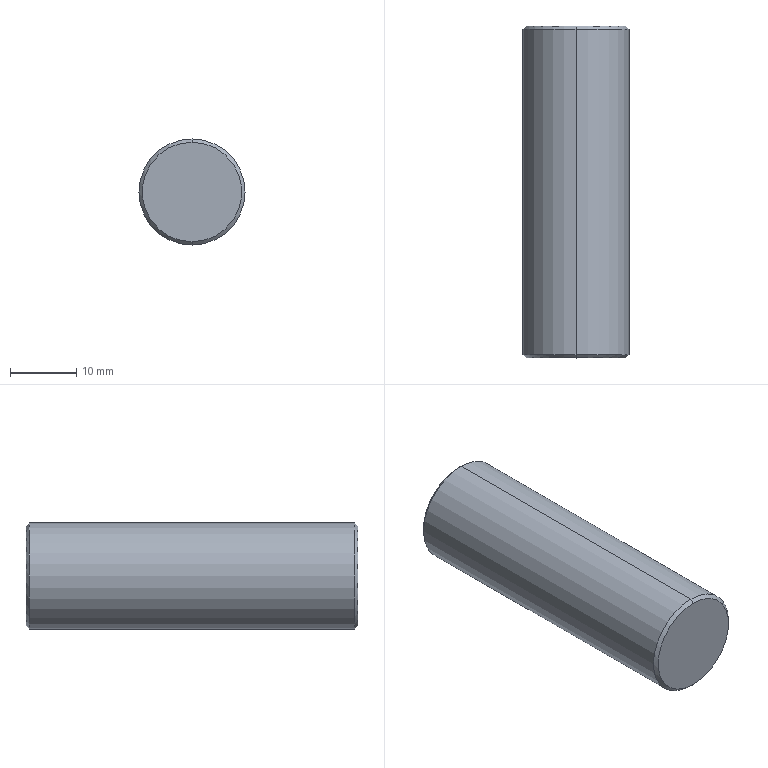Part | STEP file | PN_0011 Handle | 1 solid | 12 faces | box 16 x 50 x 16 mm | volume 9697 mm3 | cone 6 | cylinder 4 | plane 2 | commonest cylinder face diameters 5 x2 16 x2
STEP:
#1=CARTESIAN_POINT('',(0.,0.,0.));
#2=DIRECTION('',(0.,0.,1.));
#3=DIRECTION('',(1.,0.,0.));
#4=AXIS2_PLACEMENT_3D('',#1,#2,#3);
#5=CARTESIAN_POINT('',(0.,49.5,-8.));
#6=VERTEX_POINT('',#5);
#7=CARTESIAN_POINT('',(0.,49.5,8.));
#8=VERTEX_POINT('',#7);
#9=CARTESIAN_POINT('',(0.,49.5,0.));
#10=DIRECTION('',(0.,-1.,0.));
#11=DIRECTION('',(0.,0.,-1.));
#12=AXIS2_PLACEMENT_3D('',#9,#10,#11);
#13=CIRCLE('',#12,8.);
#14=CARTESIAN_POINT('',(0.,50.,0.));
#15=DIRECTION('',(0.,-1.,0.));
#16=DIRECTION('',(0.,0.,-1.));
#17=AXIS2_PLACEMENT_3D('',#14,#15,#16);
#18=CYLINDRICAL_SURFACE('',#17,8.);
#19=CARTESIAN_POINT('',(0.,0.5));
#20=DIRECTION('',(1.,0.));
#21=VECTOR('',#20,1.);
#22=LINE('',#19,#21);
#23=(GEOMETRIC_REPRESENTATION_CONTEXT(2)PARAMETRIC_REPRESENTATION_CONTEXT()REPRESENTATION_CONTEXT('',''));
#24=DEFINITIONAL_REPRESENTATION('',(#22),#23);
#25=PCURVE('',#18,#24);
#26=CARTESIAN_POINT('',(0.,49.5,0.));
#27=DIRECTION('',(0.,-1.,0.));
#28=DIRECTION('',(0.,0.,-1.));
#29=AXIS2_PLACEMENT_3D('',#26,#27,#28);
#30=CONICAL_SURFACE('',#29,8.,0.7854);
#31=CARTESIAN_POINT('',(0.,0.));
#32=DIRECTION('',(1.,0.));
#33=VECTOR('',#32,1.);
#34=LINE('',#31,#33);
#35=(GEOMETRIC_REPRESENTATION_CONTEXT(2)PARAMETRIC_REPRESENTATION_CONTEXT()REPRESENTATION_CONTEXT('',''));
#36=DEFINITIONAL_REPRESENTATION('',(#34),#35);
#37=PCURVE('',#30,#36);
#38=SURFACE_CURVE('',#13,(#25,#37),.PCURVE_S1.);
#39=EDGE_CURVE('',#6,#8,#38,.T.);
#40=ORIENTED_EDGE('',*,*,#39,.T.);
#41=CARTESIAN_POINT('',(0.,0.5,8.));
#42=VERTEX_POINT('',#41);
#43=CARTESIAN_POINT('',(0.,50.,8.));
#44=DIRECTION('',(0.,-1.,0.));
#45=VECTOR('',#44,1.);
#46=LINE('',#43,#45);
#47=CARTESIAN_POINT('',(3.142,0.));
#48=DIRECTION('',(0.,1.));
#49=VECTOR('',#48,1.);
#50=LINE('',#47,#49);
#51=(GEOMETRIC_REPRESENTATION_CONTEXT(2)PARAMETRIC_REPRESENTATION_CONTEXT()REPRESENTATION_CONTEXT('',''));
#52=DEFINITIONAL_REPRESENTATION('',(#50),#51);
#53=PCURVE('',#18,#52);
#54=CARTESIAN_POINT('',(0.,50.,0.));
#55=DIRECTION('',(0.,-1.,0.));
#56=DIRECTION('',(0.,0.,-1.));
#57=AXIS2_PLACEMENT_3D('',#54,#55,#56);
#58=CYLINDRICAL_SURFACE('',#57,8.);
#59=CARTESIAN_POINT('',(3.142,0.));
#60=DIRECTION('',(0.,1.));
#61=VECTOR('',#60,1.);
#62=LINE('',#59,#61);
#63=(GEOMETRIC_REPRESENTATION_CONTEXT(2)PARAMETRIC_REPRESENTATION_CONTEXT()REPRESENTATION_CONTEXT('',''));
#64=DEFINITIONAL_REPRESENTATION('',(#62),#63);
#65=PCURVE('',#58,#64);
#66=SURFACE_CURVE('',#46,(#53,#65),.PCURVE_S1.);
#67=EDGE_CURVE('',#8,#42,#66,.T.);
#68=ORIENTED_EDGE('',*,*,#67,.T.);
#69=CARTESIAN_POINT('',(0.,0.5,-8.));
#70=VERTEX_POINT('',#69);
#71=CARTESIAN_POINT('',(0.,0.5,0.));
#72=DIRECTION('',(0.,1.,0.));
#73=DIRECTION('',(0.,0.,-1.));
#74=AXIS2_PLACEMENT_3D('',#71,#72,#73);
#75=CIRCLE('',#74,8.);
#76=CARTESIAN_POINT('',(6.283,49.5));
#77=DIRECTION('',(-1.,0.));
#78=VECTOR('',#77,1.);
#79=LINE('',#76,#78);
#80=(GEOMETRIC_REPRESENTATION_CONTEXT(2)PARAMETRIC_REPRESENTATION_CONTEXT()REPRESENTATION_CONTEXT('',''));
#81=DEFINITIONAL_REPRESENTATION('',(#79),#80);
#82=PCURVE('',#18,#81);
#83=CARTESIAN_POINT('',(0.,0.5,0.));
#84=DIRECTION('',(0.,1.,0.));
#85=DIRECTION('',(0.,0.,1.));
#86=AXIS2_PLACEMENT_3D('',#83,#84,#85);
#87=CONICAL_SURFACE('',#86,8.,0.7854);
#88=CARTESIAN_POINT('',(-3.142,0.));
#89=DIRECTION('',(1.,0.));
#90=VECTOR('',#89,1.);
#91=LINE('',#88,#90);
#92=(GEOMETRIC_REPRESENTATION_CONTEXT(2)PARAMETRIC_REPRESENTATION_CONTEXT()REPRESENTATION_CONTEXT('',''));
#93=DEFINITIONAL_REPRESENTATION('',(#91),#92);
#94=PCURVE('',#87,#93);
#95=SURFACE_CURVE('',#75,(#82,#94),.PCURVE_S1.);
#96=EDGE_CURVE('',#42,#70,#95,.T.);
#97=ORIENTED_EDGE('',*,*,#96,.T.);
#98=CARTESIAN_POINT('',(0.,50.,-8.));
#99=DIRECTION('',(0.,-1.,0.));
#100=VECTOR('',#99,1.);
#101=LINE('',#98,#100);
#102=CARTESIAN_POINT('',(0.,0.));
#103=DIRECTION('',(0.,1.));
#104=VECTOR('',#103,1.);
#105=LINE('',#102,#104);
#106=(GEOMETRIC_REPRESENTATION_CONTEXT(2)PARAMETRIC_REPRESENTATION_CONTEXT()REPRESENTATION_CONTEXT('',''));
#107=DEFINITIONAL_REPRESENTATION('',(#105),#106);
#108=PCURVE('',#18,#107);
#109=CARTESIAN_POINT('',(6.283,0.));
#110=DIRECTION('',(0.,1.));
#111=VECTOR('',#110,1.);
#112=LINE('',#109,#111);
#113=(GEOMETRIC_REPRESENTATION_CONTEXT(2)PARAMETRIC_REPRESENTATION_CONTEXT()REPRESENTATION_CONTEXT('',''));
#114=DEFINITIONAL_REPRESENTATION('',(#112),#113);
#115=PCURVE('',#58,#114);
#116=SURFACE_CURVE('',#101,(#108,#115),.PCURVE_S1.);
#117=EDGE_CURVE('',#6,#70,#116,.T.);
#118=ORIENTED_EDGE('',*,*,#117,.F.);
#119=EDGE_LOOP('',(#40,#68,#97,#118));
#120=FACE_BOUND('',#119,.T.);
#121=ADVANCED_FACE('',(#120),#18,.T.);
#122=CARTESIAN_POINT('',(0.,0.,7.5));
#123=VERTEX_POINT('',#122);
#124=CARTESIAN_POINT('',(0.,0.,-7.5));
#125=VERTEX_POINT('',#124);
#126=CARTESIAN_POINT('',(0.,0.,0.));
#127=DIRECTION('',(0.,1.,0.));
#128=DIRECTION('',(0.,0.,1.));
#129=AXIS2_PLACEMENT_3D('',#126,#127,#128);
#130=CIRCLE('',#129,7.5);
#131=CARTESIAN_POINT('',(0.,-0.5));
#132=DIRECTION('',(1.,0.));
#133=VECTOR('',#132,1.);
#134=LINE('',#131,#133);
#135=(GEOMETRIC_REPRESENTATION_CONTEXT(2)PARAMETRIC_REPRESENTATION_CONTEXT()REPRESENTATION_CONTEXT('',''));
#136=DEFINITIONAL_REPRESENTATION('',(#134),#135);
#137=PCURVE('',#87,#136);
#138=CARTESIAN_POINT('',(0.,0.,0.));
#139=DIRECTION('',(0.,1.,0.));
#140=DIRECTION('',(0.,0.,1.));
#141=AXIS2_PLACEMENT_3D('',#138,#139,#140);
#142=PLANE('',#141);
#143=CARTESIAN_POINT('',(0.,0.));
#144=DIRECTION('',(1.,0.));
#145=AXIS2_PLACEMENT_2D('',#143,#144);
#146=CIRCLE('',#145,7.5);
#147=(GEOMETRIC_REPRESENTATION_CONTEXT(2)PARAMETRIC_REPRESENTATION_CONTEXT()REPRESENTATION_CONTEXT('',''));
#148=DEFINITIONAL_REPRESENTATION('',(#146),#147);
#149=PCURVE('',#142,#148);
#150=SURFACE_CURVE('',#130,(#137,#149),.PCURVE_S1.);
#151=EDGE_CURVE('',#123,#125,#150,.T.);
#152=ORIENTED_EDGE('',*,*,#151,.T.);
#153=CARTESIAN_POINT('',(0.,0.5,-8.));
#154=DIRECTION('',(0.,0.7071,-0.7071));
#155=VECTOR('',#154,1.);
#156=LINE('',#153,#155);
#157=CARTESIAN_POINT('',(3.142,0.));
#158=DIRECTION('',(0.,1.));
#159=VECTOR('',#158,1.);
#160=LINE('',#157,#159);
#161=(GEOMETRIC_REPRESENTATION_CONTEXT(2)PARAMETRIC_REPRESENTATION_CONTEXT()REPRESENTATION_CONTEXT('',''));
#162=DEFINITIONAL_REPRESENTATION('',(#160),#161);
#163=PCURVE('',#87,#162);
#164=CARTESIAN_POINT('',(0.,0.5,0.));
#165=DIRECTION('',(0.,1.,0.));
#166=DIRECTION('',(0.,0.,1.));
#167=AXIS2_PLACEMENT_3D('',#164,#165,#166);
#168=CONICAL_SURFACE('',#167,8.,0.7854);
#169=CARTESIAN_POINT('',(3.142,0.));
#170=DIRECTION('',(0.,1.));
#171=VECTOR('',#170,1.);
#172=LINE('',#169,#171);
#173=(GEOMETRIC_REPRESENTATION_CONTEXT(2)PARAMETRIC_REPRESENTATION_CONTEXT()REPRESENTATION_CONTEXT('',''));
#174=DEFINITIONAL_REPRESENTATION('',(#172),#173);
#175=PCURVE('',#168,#174);
#176=SURFACE_CURVE('',#156,(#163,#175),.PCURVE_S1.);
#177=EDGE_CURVE('',#125,#70,#176,.T.);
#178=ORIENTED_EDGE('',*,*,#177,.T.);
#179=ORIENTED_EDGE('',*,*,#96,.F.);
#180=CARTESIAN_POINT('',(0.,0.5,8.));
#181=DIRECTION('',(0.,0.7071,0.7071));
#182=VECTOR('',#181,1.);
#183=LINE('',#180,#182);
#184=CARTESIAN_POINT('',(0.,0.));
#185=DIRECTION('',(0.,1.));
#186=VECTOR('',#185,1.);
#187=LINE('',#184,#186);
#188=(GEOMETRIC_REPRESENTATION_CONTEXT(2)PARAMETRIC_REPRESENTATION_CONTEXT()REPRESENTATION_CONTEXT('',''));
#189=DEFINITIONAL_REPRESENTATION('',(#187),#188);
#190=PCURVE('',#87,#189);
#191=CARTESIAN_POINT('',(6.283,0.));
#192=DIRECTION('',(0.,1.));
#193=VECTOR('',#192,1.);
#194=LINE('',#191,#193);
#195=(GEOMETRIC_REPRESENTATION_CONTEXT(2)PARAMETRIC_REPRESENTATION_CONTEXT()REPRESENTATION_CONTEXT('',''));
#196=DEFINITIONAL_REPRESENTATION('',(#194),#195);
#197=PCURVE('',#168,#196);
#198=SURFACE_CURVE('',#183,(#190,#197),.PCURVE_S1.);
#199=EDGE_CURVE('',#123,#42,#198,.T.);
#200=ORIENTED_EDGE('',*,*,#199,.F.);
#201=EDGE_LOOP('',(#152,#178,#179,#200));
#202=FACE_BOUND('',#201,.T.);
#203=ADVANCED_FACE('',(#202),#87,.T.);
#204=CARTESIAN_POINT('',(0.,50.,-7.5));
#205=VERTEX_POINT('',#204);
#206=CARTESIAN_POINT('',(0.,50.,7.5));
#207=VERTEX_POINT('',#206);
#208=CARTESIAN_POINT('',(0.,50.,0.));
#209=DIRECTION('',(0.,-1.,0.));
#210=DIRECTION('',(0.,0.,-1.));
#211=AXIS2_PLACEMENT_3D('',#208,#209,#210);
#212=CIRCLE('',#211,7.5);
#213=CARTESIAN_POINT('',(0.,-0.5));
#214=DIRECTION('',(1.,0.));
#215=VECTOR('',#214,1.);
#216=LINE('',#213,#215);
#217=(GEOMETRIC_REPRESENTATION_CONTEXT(2)PARAMETRIC_REPRESENTATION_CONTEXT()REPRESENTATION_CONTEXT('',''));
#218=DEFINITIONAL_REPRESENTATION('',(#216),#217);
#219=PCURVE('',#30,#218);
#220=CARTESIAN_POINT('',(0.,50.,0.));
#221=DIRECTION('',(0.,1.,0.));
#222=DIRECTION('',(0.,0.,1.));
#223=AXIS2_PLACEMENT_3D('',#220,#221,#222);
#224=PLANE('',#223);
#225=CARTESIAN_POINT('',(-7.5,0.));
#226=CARTESIAN_POINT('',(-7.5,12.99));
#227=CARTESIAN_POINT('',(3.75,6.495));
#228=CARTESIAN_POINT('',(15.,0.));
#229=CARTESIAN_POINT('',(3.75,-6.495));
#230=CARTESIAN_POINT('',(-7.5,-12.99));
#231=CARTESIAN_POINT('',(-7.5,0.));
#232=(BOUNDED_CURVE()B_SPLINE_CURVE(2,(#225,#226,#227,#228,#229,#230,#231),.UNSPECIFIED.,.T.,.F.)B_SPLINE_CURVE_WITH_KNOTS((1,2,2,2,2,1),(-2.094,0.,2.094,4.189,6.283,8.378),.UNSPECIFIED.)CURVE()GEOMETRIC_REPRESENTATION_ITEM()RATIONAL_B_SPLINE_CURVE((1.,0.5,1.,0.5,1.,0.5,1.))REPRESENTATION_ITEM(''));
#233=(GEOMETRIC_REPRESENTATION_CONTEXT(2)PARAMETRIC_REPRESENTATION_CONTEXT()REPRESENTATION_CONTEXT('',''));
#234=DEFINITIONAL_REPRESENTATION('',(#232),#233);
#235=PCURVE('',#224,#234);
#236=SURFACE_CURVE('',#212,(#219,#235),.PCURVE_S1.);
#237=EDGE_CURVE('',#205,#207,#236,.T.);
#238=ORIENTED_EDGE('',*,*,#237,.T.);
#239=CARTESIAN_POINT('',(0.,49.5,8.));
#240=DIRECTION('',(0.,-0.7071,0.7071));
#241=VECTOR('',#240,1.);
#242=LINE('',#239,#241);
#243=CARTESIAN_POINT('',(3.142,0.));
#244=DIRECTION('',(0.,1.));
#245=VECTOR('',#244,1.);
#246=LINE('',#243,#245);
#247=(GEOMETRIC_REPRESENTATION_CONTEXT(2)PARAMETRIC_REPRESENTATION_CONTEXT()REPRESENTATION_CONTEXT('',''));
#248=DEFINITIONAL_REPRESENTATION('',(#246),#247);
#249=PCURVE('',#30,#248);
#250=CARTESIAN_POINT('',(0.,49.5,0.));
#251=DIRECTION('',(0.,-1.,0.));
#252=DIRECTION('',(0.,0.,-1.));
#253=AXIS2_PLACEMENT_3D('',#250,#251,#252);
#254=CONICAL_SURFACE('',#253,8.,0.7854);
#255=CARTESIAN_POINT('',(3.142,0.));
#256=DIRECTION('',(0.,1.));
#257=VECTOR('',#256,1.);
#258=LINE('',#255,#257);
#259=(GEOMETRIC_REPRESENTATION_CONTEXT(2)PARAMETRIC_REPRESENTATION_CONTEXT()REPRESENTATION_CONTEXT('',''));
#260=DEFINITIONAL_REPRESENTATION('',(#258),#259);
#261=PCURVE('',#254,#260);
#262=SURFACE_CURVE('',#242,(#249,#261),.PCURVE_S1.);
#263=EDGE_CURVE('',#207,#8,#262,.T.);
#264=ORIENTED_EDGE('',*,*,#263,.T.);
#265=ORIENTED_EDGE('',*,*,#39,.F.);
#266=CARTESIAN_POINT('',(0.,49.5,-8.));
#267=DIRECTION('',(0.,-0.7071,-0.7071));
#268=VECTOR('',#267,1.);
#269=LINE('',#266,#268);
#270=CARTESIAN_POINT('',(0.,0.));
#271=DIRECTION('',(0.,1.));
#272=VECTOR('',#271,1.);
#273=LINE('',#270,#272);
#274=(GEOMETRIC_REPRESENTATION_CONTEXT(2)PARAMETRIC_REPRESENTATION_CONTEXT()REPRESENTATION_CONTEXT('',''));
#275=DEFINITIONAL_REPRESENTATION('',(#273),#274);
#276=PCURVE('',#30,#275);
#277=CARTESIAN_POINT('',(6.283,0.));
#278=DIRECTION('',(0.,1.));
#279=VECTOR('',#278,1.);
#280=LINE('',#277,#279);
#281=(GEOMETRIC_REPRESENTATION_CONTEXT(2)PARAMETRIC_REPRESENTATION_CONTEXT()REPRESENTATION_CONTEXT('',''));
#282=DEFINITIONAL_REPRESENTATION('',(#280),#281);
#283=PCURVE('',#254,#282);
#284=SURFACE_CURVE('',#269,(#276,#283),.PCURVE_S1.);
#285=EDGE_CURVE('',#205,#6,#284,.T.);
#286=ORIENTED_EDGE('',*,*,#285,.F.);
#287=EDGE_LOOP('',(#238,#264,#265,#286));
#288=FACE_BOUND('',#287,.T.);
#289=ADVANCED_FACE('',(#288),#30,.T.);
#290=CARTESIAN_POINT('',(0.,33.,2.5));
#291=VERTEX_POINT('',#290);
#292=CARTESIAN_POINT('',(0.,50.,2.5));
#293=VERTEX_POINT('',#292);
#294=CARTESIAN_POINT('',(0.,50.,2.5));
#295=DIRECTION('',(0.,1.,0.));
#296=VECTOR('',#295,1.);
#297=LINE('',#294,#296);
#298=CARTESIAN_POINT('',(0.,50.,0.));
#299=DIRECTION('',(0.,1.,0.));
#300=DIRECTION('',(0.,0.,1.));
#301=AXIS2_PLACEMENT_3D('',#298,#299,#300);
#302=CYLINDRICAL_SURFACE('',#301,2.5);
#303=CARTESIAN_POINT('',(6.283,0.));
#304=DIRECTION('',(0.,1.));
#305=VECTOR('',#304,1.);
#306=LINE('',#303,#305);
#307=(GEOMETRIC_REPRESENTATION_CONTEXT(2)PARAMETRIC_REPRESENTATION_CONTEXT()REPRESENTATION_CONTEXT('',''));
#308=DEFINITIONAL_REPRESENTATION('',(#306),#307);
#309=PCURVE('',#302,#308);
#310=CARTESIAN_POINT('',(0.,50.,0.));
#311=DIRECTION('',(0.,1.,0.));
#312=DIRECTION('',(0.,0.,1.));
#313=AXIS2_PLACEMENT_3D('',#310,#311,#312);
#314=CYLINDRICAL_SURFACE('',#313,2.5);
#315=CARTESIAN_POINT('',(0.,0.));
#316=DIRECTION('',(0.,1.));
#317=VECTOR('',#316,1.);
#318=LINE('',#315,#317);
#319=(GEOMETRIC_REPRESENTATION_CONTEXT(2)PARAMETRIC_REPRESENTATION_CONTEXT()REPRESENTATION_CONTEXT('',''));
#320=DEFINITIONAL_REPRESENTATION('',(#318),#319);
#321=PCURVE('',#314,#320);
#322=SURFACE_CURVE('',#297,(#309,#321),.PCURVE_S1.);
#323=EDGE_CURVE('',#291,#293,#322,.T.);
#324=ORIENTED_EDGE('',*,*,#323,.T.);
#325=CARTESIAN_POINT('',(0.,50.,-2.5));
#326=VERTEX_POINT('',#325);
#327=CARTESIAN_POINT('',(0.,50.,0.));
#328=DIRECTION('',(0.,-1.,0.));
#329=DIRECTION('',(0.,0.,1.));
#330=AXIS2_PLACEMENT_3D('',#327,#328,#329);
#331=CIRCLE('',#330,2.5);
#332=CARTESIAN_POINT('',(6.283,0.));
#333=DIRECTION('',(-1.,0.));
#334=VECTOR('',#333,1.);
#335=LINE('',#332,#334);
#336=(GEOMETRIC_REPRESENTATION_CONTEXT(2)PARAMETRIC_REPRESENTATION_CONTEXT()REPRESENTATION_CONTEXT('',''));
#337=DEFINITIONAL_REPRESENTATION('',(#335),#336);
#338=PCURVE('',#302,#337);
#339=CARTESIAN_POINT('',(2.5,0.));
#340=CARTESIAN_POINT('',(2.5,-4.33));
#341=CARTESIAN_POINT('',(-1.25,-2.165));
#342=CARTESIAN_POINT('',(-5.,0.));
#343=CARTESIAN_POINT('',(-1.25,2.165));
#344=CARTESIAN_POINT('',(2.5,4.33));
#345=CARTESIAN_POINT('',(2.5,0.));
#346=(BOUNDED_CURVE()B_SPLINE_CURVE(2,(#339,#340,#341,#342,#343,#344,#345),.UNSPECIFIED.,.T.,.F.)B_SPLINE_CURVE_WITH_KNOTS((1,2,2,2,2,1),(-2.094,0.,2.094,4.189,6.283,8.378),.UNSPECIFIED.)CURVE()GEOMETRIC_REPRESENTATION_ITEM()RATIONAL_B_SPLINE_CURVE((1.,0.5,1.,0.5,1.,0.5,1.))REPRESENTATION_ITEM(''));
#347=(GEOMETRIC_REPRESENTATION_CONTEXT(2)PARAMETRIC_REPRESENTATION_CONTEXT()REPRESENTATION_CONTEXT('',''));
#348=DEFINITIONAL_REPRESENTATION('',(#346),#347);
#349=PCURVE('',#224,#348);
#350=SURFACE_CURVE('',#331,(#338,#349),.PCURVE_S1.);
#351=EDGE_CURVE('',#293,#326,#350,.T.);
#352=ORIENTED_EDGE('',*,*,#351,.T.);
#353=CARTESIAN_POINT('',(0.,33.,-2.5));
#354=VERTEX_POINT('',#353);
#355=CARTESIAN_POINT('',(0.,50.,-2.5));
#356=DIRECTION('',(0.,1.,0.));
#357=VECTOR('',#356,1.);
#358=LINE('',#355,#357);
#359=CARTESIAN_POINT('',(3.142,0.));
#360=DIRECTION('',(0.,1.));
#361=VECTOR('',#360,1.);
#362=LINE('',#359,#361);
#363=(GEOMETRIC_REPRESENTATION_CONTEXT(2)PARAMETRIC_REPRESENTATION_CONTEXT()REPRESENTATION_CONTEXT('',''));
#364=DEFINITIONAL_REPRESENTATION('',(#362),#363);
#365=PCURVE('',#302,#364);
#366=CARTESIAN_POINT('',(3.142,0.));
#367=DIRECTION('',(0.,1.));
#368=VECTOR('',#367,1.);
#369=LINE('',#366,#368);
#370=(GEOMETRIC_REPRESENTATION_CONTEXT(2)PARAMETRIC_REPRESENTATION_CONTEXT()REPRESENTATION_CONTEXT('',''));
#371=DEFINITIONAL_REPRESENTATION('',(#369),#370);
#372=PCURVE('',#314,#371);
#373=SURFACE_CURVE('',#358,(#365,#372),.PCURVE_S1.);
#374=EDGE_CURVE('',#354,#326,#373,.T.);
#375=ORIENTED_EDGE('',*,*,#374,.F.);
#376=CARTESIAN_POINT('',(0.,33.,0.));
#377=DIRECTION('',(0.,1.,0.));
#378=DIRECTION('',(0.,0.,1.));
#379=AXIS2_PLACEMENT_3D('',#376,#377,#378);
#380=CIRCLE('',#379,2.5);
#381=CARTESIAN_POINT('',(0.,-17.));
#382=DIRECTION('',(1.,0.));
#383=VECTOR('',#382,1.);
#384=LINE('',#381,#383);
#385=(GEOMETRIC_REPRESENTATION_CONTEXT(2)PARAMETRIC_REPRESENTATION_CONTEXT()REPRESENTATION_CONTEXT('',''));
#386=DEFINITIONAL_REPRESENTATION('',(#384),#385);
#387=PCURVE('',#302,#386);
#388=CARTESIAN_POINT('',(0.,33.,0.));
#389=DIRECTION('',(0.,1.,0.));
#390=DIRECTION('',(0.,0.,1.));
#391=AXIS2_PLACEMENT_3D('',#388,#389,#390);
#392=CONICAL_SURFACE('',#391,2.5,1.03);
#393=CARTESIAN_POINT('',(0.,0.));
#394=DIRECTION('',(1.,0.));
#395=VECTOR('',#394,1.);
#396=LINE('',#393,#395);
#397=(GEOMETRIC_REPRESENTATION_CONTEXT(2)PARAMETRIC_REPRESENTATION_CONTEXT()REPRESENTATION_CONTEXT('',''));
#398=DEFINITIONAL_REPRESENTATION('',(#396),#397);
#399=PCURVE('',#392,#398);
#400=SURFACE_CURVE('',#380,(#387,#399),.PCURVE_S1.);
#401=EDGE_CURVE('',#354,#291,#400,.T.);
#402=ORIENTED_EDGE('',*,*,#401,.T.);
#403=EDGE_LOOP('',(#324,#352,#375,#402));
#404=FACE_BOUND('',#403,.F.);
#405=ADVANCED_FACE('',(#404),#302,.F.);
#406=ORIENTED_EDGE('',*,*,#401,.F.);
#407=CARTESIAN_POINT('',(0.,31.498,0.));
#408=VERTEX_POINT('',#407);
#409=CARTESIAN_POINT('',(0.,33.,-2.5));
#410=DIRECTION('',(0.,0.515,-0.8572));
#411=VECTOR('',#410,1.);
#412=LINE('',#409,#411);
#413=CARTESIAN_POINT('',(3.142,0.));
#414=DIRECTION('',(0.,1.));
#415=VECTOR('',#414,1.);
#416=LINE('',#413,#415);
#417=(GEOMETRIC_REPRESENTATION_CONTEXT(2)PARAMETRIC_REPRESENTATION_CONTEXT()REPRESENTATION_CONTEXT('',''));
#418=DEFINITIONAL_REPRESENTATION('',(#416),#417);
#419=PCURVE('',#392,#418);
#420=CARTESIAN_POINT('',(0.,33.,0.));
#421=DIRECTION('',(0.,1.,0.));
#422=DIRECTION('',(0.,0.,1.));
#423=AXIS2_PLACEMENT_3D('',#420,#421,#422);
#424=CONICAL_SURFACE('',#423,2.5,1.03);
#425=CARTESIAN_POINT('',(3.142,0.));
#426=DIRECTION('',(0.,1.));
#427=VECTOR('',#426,1.);
#428=LINE('',#425,#427);
#429=(GEOMETRIC_REPRESENTATION_CONTEXT(2)PARAMETRIC_REPRESENTATION_CONTEXT()REPRESENTATION_CONTEXT('',''));
#430=DEFINITIONAL_REPRESENTATION('',(#428),#429);
#431=PCURVE('',#424,#430);
#432=SURFACE_CURVE('',#412,(#419,#431),.PCURVE_S1.);
#433=EDGE_CURVE('',#408,#354,#432,.T.);
#434=ORIENTED_EDGE('',*,*,#433,.F.);
#435=CARTESIAN_POINT('',(0.,33.,2.5));
#436=DIRECTION('',(0.,0.515,0.8572));
#437=VECTOR('',#436,1.);
#438=LINE('',#435,#437);
#439=CARTESIAN_POINT('',(6.283,0.));
#440=DIRECTION('',(0.,1.));
#441=VECTOR('',#440,1.);
#442=LINE('',#439,#441);
#443=(GEOMETRIC_REPRESENTATION_CONTEXT(2)PARAMETRIC_REPRESENTATION_CONTEXT()REPRESENTATION_CONTEXT('',''));
#444=DEFINITIONAL_REPRESENTATION('',(#442),#443);
#445=PCURVE('',#392,#444);
#446=CARTESIAN_POINT('',(0.,0.));
#447=DIRECTION('',(0.,1.));
#448=VECTOR('',#447,1.);
#449=LINE('',#446,#448);
#450=(GEOMETRIC_REPRESENTATION_CONTEXT(2)PARAMETRIC_REPRESENTATION_CONTEXT()REPRESENTATION_CONTEXT('',''));
#451=DEFINITIONAL_REPRESENTATION('',(#449),#450);
#452=PCURVE('',#424,#451);
#453=SURFACE_CURVE('',#438,(#445,#452),.PCURVE_S1.);
#454=EDGE_CURVE('',#408,#291,#453,.T.);
#455=ORIENTED_EDGE('',*,*,#454,.T.);
#456=EDGE_LOOP('',(#406,#434,#455));
#457=FACE_BOUND('',#456,.F.);
#458=ADVANCED_FACE('',(#457),#392,.F.);
#459=ORIENTED_EDGE('',*,*,#67,.F.);
#460=CARTESIAN_POINT('',(0.,49.5,0.));
#461=DIRECTION('',(0.,-1.,0.));
#462=DIRECTION('',(0.,0.,-1.));
#463=AXIS2_PLACEMENT_3D('',#460,#461,#462);
#464=CIRCLE('',#463,8.);
#465=CARTESIAN_POINT('',(0.,0.5));
#466=DIRECTION('',(1.,0.));
#467=VECTOR('',#466,1.);
#468=LINE('',#465,#467);
#469=(GEOMETRIC_REPRESENTATION_CONTEXT(2)PARAMETRIC_REPRESENTATION_CONTEXT()REPRESENTATION_CONTEXT('',''));
#470=DEFINITIONAL_REPRESENTATION('',(#468),#469);
#471=PCURVE('',#58,#470);
#472=CARTESIAN_POINT('',(0.,0.));
#473=DIRECTION('',(1.,0.));
#474=VECTOR('',#473,1.);
#475=LINE('',#472,#474);
#476=(GEOMETRIC_REPRESENTATION_CONTEXT(2)PARAMETRIC_REPRESENTATION_CONTEXT()REPRESENTATION_CONTEXT('',''));
#477=DEFINITIONAL_REPRESENTATION('',(#475),#476);
#478=PCURVE('',#254,#477);
#479=SURFACE_CURVE('',#464,(#471,#478),.PCURVE_S1.);
#480=EDGE_CURVE('',#8,#6,#479,.T.);
#481=ORIENTED_EDGE('',*,*,#480,.T.);
#482=ORIENTED_EDGE('',*,*,#117,.T.);
#483=CARTESIAN_POINT('',(0.,0.5,0.));
#484=DIRECTION('',(0.,1.,0.));
#485=DIRECTION('',(0.,0.,-1.));
#486=AXIS2_PLACEMENT_3D('',#483,#484,#485);
#487=CIRCLE('',#486,8.);
#488=CARTESIAN_POINT('',(6.283,49.5));
#489=DIRECTION('',(-1.,0.));
#490=VECTOR('',#489,1.);
#491=LINE('',#488,#490);
#492=(GEOMETRIC_REPRESENTATION_CONTEXT(2)PARAMETRIC_REPRESENTATION_CONTEXT()REPRESENTATION_CONTEXT('',''));
#493=DEFINITIONAL_REPRESENTATION('',(#491),#492);
#494=PCURVE('',#58,#493);
#495=CARTESIAN_POINT('',(3.142,0.));
#496=DIRECTION('',(1.,0.));
#497=VECTOR('',#496,1.);
#498=LINE('',#495,#497);
#499=(GEOMETRIC_REPRESENTATION_CONTEXT(2)PARAMETRIC_REPRESENTATION_CONTEXT()REPRESENTATION_CONTEXT('',''));
#500=DEFINITIONAL_REPRESENTATION('',(#498),#499);
#501=PCURVE('',#168,#500);
#502=SURFACE_CURVE('',#487,(#494,#501),.PCURVE_S1.);
#503=EDGE_CURVE('',#70,#42,#502,.T.);
#504=ORIENTED_EDGE('',*,*,#503,.T.);
#505=EDGE_LOOP('',(#459,#481,#482,#504));
#506=FACE_BOUND('',#505,.T.);
#507=ADVANCED_FACE('',(#506),#58,.T.);
#508=ORIENTED_EDGE('',*,*,#177,.F.);
#509=CARTESIAN_POINT('',(0.,0.,0.));
#510=DIRECTION('',(0.,1.,0.));
#511=DIRECTION('',(0.,0.,1.));
#512=AXIS2_PLACEMENT_3D('',#509,#510,#511);
#513=CIRCLE('',#512,7.5);
#514=CARTESIAN_POINT('',(0.,-0.5));
#515=DIRECTION('',(1.,0.));
#516=VECTOR('',#515,1.);
#517=LINE('',#514,#516);
#518=(GEOMETRIC_REPRESENTATION_CONTEXT(2)PARAMETRIC_REPRESENTATION_CONTEXT()REPRESENTATION_CONTEXT('',''));
#519=DEFINITIONAL_REPRESENTATION('',(#517),#518);
#520=PCURVE('',#168,#519);
#521=CARTESIAN_POINT('',(0.,0.));
#522=DIRECTION('',(1.,0.));
#523=AXIS2_PLACEMENT_2D('',#521,#522);
#524=CIRCLE('',#523,7.5);
#525=(GEOMETRIC_REPRESENTATION_CONTEXT(2)PARAMETRIC_REPRESENTATION_CONTEXT()REPRESENTATION_CONTEXT('',''));
#526=DEFINITIONAL_REPRESENTATION('',(#524),#525);
#527=PCURVE('',#142,#526);
#528=SURFACE_CURVE('',#513,(#520,#527),.PCURVE_S1.);
#529=EDGE_CURVE('',#125,#123,#528,.T.);
#530=ORIENTED_EDGE('',*,*,#529,.T.);
#531=ORIENTED_EDGE('',*,*,#199,.T.);
#532=ORIENTED_EDGE('',*,*,#503,.F.);
#533=EDGE_LOOP('',(#508,#530,#531,#532));
#534=FACE_BOUND('',#533,.T.);
#535=ADVANCED_FACE('',(#534),#168,.T.);
#536=ORIENTED_EDGE('',*,*,#263,.F.);
#537=CARTESIAN_POINT('',(0.,50.,0.));
#538=DIRECTION('',(0.,-1.,0.));
#539=DIRECTION('',(0.,0.,-1.));
#540=AXIS2_PLACEMENT_3D('',#537,#538,#539);
#541=CIRCLE('',#540,7.5);
#542=CARTESIAN_POINT('',(0.,-0.5));
#543=DIRECTION('',(1.,0.));
#544=VECTOR('',#543,1.);
#545=LINE('',#542,#544);
#546=(GEOMETRIC_REPRESENTATION_CONTEXT(2)PARAMETRIC_REPRESENTATION_CONTEXT()REPRESENTATION_CONTEXT('',''));
#547=DEFINITIONAL_REPRESENTATION('',(#545),#546);
#548=PCURVE('',#254,#547);
#549=CARTESIAN_POINT('',(-7.5,0.));
#550=CARTESIAN_POINT('',(-7.5,12.99));
#551=CARTESIAN_POINT('',(3.75,6.495));
#552=CARTESIAN_POINT('',(15.,0.));
#553=CARTESIAN_POINT('',(3.75,-6.495));
#554=CARTESIAN_POINT('',(-7.5,-12.99));
#555=CARTESIAN_POINT('',(-7.5,0.));
#556=(BOUNDED_CURVE()B_SPLINE_CURVE(2,(#549,#550,#551,#552,#553,#554,#555),.UNSPECIFIED.,.T.,.F.)B_SPLINE_CURVE_WITH_KNOTS((1,2,2,2,2,1),(-2.094,0.,2.094,4.189,6.283,8.378),.UNSPECIFIED.)CURVE()GEOMETRIC_REPRESENTATION_ITEM()RATIONAL_B_SPLINE_CURVE((1.,0.5,1.,0.5,1.,0.5,1.))REPRESENTATION_ITEM(''));
#557=(GEOMETRIC_REPRESENTATION_CONTEXT(2)PARAMETRIC_REPRESENTATION_CONTEXT()REPRESENTATION_CONTEXT('',''));
#558=DEFINITIONAL_REPRESENTATION('',(#556),#557);
#559=PCURVE('',#224,#558);
#560=SURFACE_CURVE('',#541,(#548,#559),.PCURVE_S1.);
#561=EDGE_CURVE('',#207,#205,#560,.T.);
#562=ORIENTED_EDGE('',*,*,#561,.T.);
#563=ORIENTED_EDGE('',*,*,#285,.T.);
#564=ORIENTED_EDGE('',*,*,#480,.F.);
#565=EDGE_LOOP('',(#536,#562,#563,#564));
#566=FACE_BOUND('',#565,.T.);
#567=ADVANCED_FACE('',(#566),#254,.T.);
#568=ORIENTED_EDGE('',*,*,#151,.F.);
#569=ORIENTED_EDGE('',*,*,#529,.F.);
#570=EDGE_LOOP('',(#568,#569));
#571=FACE_BOUND('',#570,.T.);
#572=ADVANCED_FACE('',(#571),#142,.F.);
#573=ORIENTED_EDGE('',*,*,#237,.F.);
#574=ORIENTED_EDGE('',*,*,#561,.F.);
#575=EDGE_LOOP('',(#573,#574));
#576=FACE_BOUND('',#575,.T.);
#577=ORIENTED_EDGE('',*,*,#351,.T.);
#578=CARTESIAN_POINT('',(0.,50.,0.));
#579=DIRECTION('',(0.,-1.,0.));
#580=DIRECTION('',(0.,0.,1.));
#581=AXIS2_PLACEMENT_3D('',#578,#579,#580);
#582=CIRCLE('',#581,2.5);
#583=CARTESIAN_POINT('',(2.5,0.));
#584=CARTESIAN_POINT('',(2.5,-4.33));
#585=CARTESIAN_POINT('',(-1.25,-2.165));
#586=CARTESIAN_POINT('',(-5.,0.));
#587=CARTESIAN_POINT('',(-1.25,2.165));
#588=CARTESIAN_POINT('',(2.5,4.33));
#589=CARTESIAN_POINT('',(2.5,0.));
#590=(BOUNDED_CURVE()B_SPLINE_CURVE(2,(#583,#584,#585,#586,#587,#588,#589),.UNSPECIFIED.,.T.,.F.)B_SPLINE_CURVE_WITH_KNOTS((1,2,2,2,2,1),(-2.094,0.,2.094,4.189,6.283,8.378),.UNSPECIFIED.)CURVE()GEOMETRIC_REPRESENTATION_ITEM()RATIONAL_B_SPLINE_CURVE((1.,0.5,1.,0.5,1.,0.5,1.))REPRESENTATION_ITEM(''));
#591=(GEOMETRIC_REPRESENTATION_CONTEXT(2)PARAMETRIC_REPRESENTATION_CONTEXT()REPRESENTATION_CONTEXT('',''));
#592=DEFINITIONAL_REPRESENTATION('',(#590),#591);
#593=PCURVE('',#224,#592);
#594=CARTESIAN_POINT('',(6.283,0.));
#595=DIRECTION('',(-1.,0.));
#596=VECTOR('',#595,1.);
#597=LINE('',#594,#596);
#598=(GEOMETRIC_REPRESENTATION_CONTEXT(2)PARAMETRIC_REPRESENTATION_CONTEXT()REPRESENTATION_CONTEXT('',''));
#599=DEFINITIONAL_REPRESENTATION('',(#597),#598);
#600=PCURVE('',#314,#599);
#601=SURFACE_CURVE('',#582,(#593,#600),.PCURVE_S1.);
#602=EDGE_CURVE('',#326,#293,#601,.T.);
#603=ORIENTED_EDGE('',*,*,#602,.T.);
#604=EDGE_LOOP('',(#577,#603));
#605=FACE_BOUND('',#604,.T.);
#606=ADVANCED_FACE('',(#576,#605),#224,.T.);
#607=ORIENTED_EDGE('',*,*,#602,.T.);
#608=ORIENTED_EDGE('',*,*,#323,.F.);
#609=CARTESIAN_POINT('',(0.,33.,0.));
#610=DIRECTION('',(0.,1.,0.));
#611=DIRECTION('',(0.,0.,1.));
#612=AXIS2_PLACEMENT_3D('',#609,#610,#611);
#613=CIRCLE('',#612,2.5);
#614=CARTESIAN_POINT('',(0.,-17.));
#615=DIRECTION('',(1.,0.));
#616=VECTOR('',#615,1.);
#617=LINE('',#614,#616);
#618=(GEOMETRIC_REPRESENTATION_CONTEXT(2)PARAMETRIC_REPRESENTATION_CONTEXT()REPRESENTATION_CONTEXT('',''));
#619=DEFINITIONAL_REPRESENTATION('',(#617),#618);
#620=PCURVE('',#314,#619);
#621=CARTESIAN_POINT('',(0.,0.));
#622=DIRECTION('',(1.,0.));
#623=VECTOR('',#622,1.);
#624=LINE('',#621,#623);
#625=(GEOMETRIC_REPRESENTATION_CONTEXT(2)PARAMETRIC_REPRESENTATION_CONTEXT()REPRESENTATION_CONTEXT('',''));
#626=DEFINITIONAL_REPRESENTATION('',(#624),#625);
#627=PCURVE('',#424,#626);
#628=SURFACE_CURVE('',#613,(#620,#627),.PCURVE_S1.);
#629=EDGE_CURVE('',#291,#354,#628,.T.);
#630=ORIENTED_EDGE('',*,*,#629,.T.);
#631=ORIENTED_EDGE('',*,*,#374,.T.);
#632=EDGE_LOOP('',(#607,#608,#630,#631));
#633=FACE_BOUND('',#632,.F.);
#634=ADVANCED_FACE('',(#633),#314,.F.);
#635=ORIENTED_EDGE('',*,*,#629,.F.);
#636=ORIENTED_EDGE('',*,*,#454,.F.);
#637=ORIENTED_EDGE('',*,*,#433,.T.);
#638=EDGE_LOOP('',(#635,#636,#637));
#639=FACE_BOUND('',#638,.F.);
#640=ADVANCED_FACE('',(#639),#424,.F.);
#641=CLOSED_SHELL('',(#121,#203,#289,#405,#458,#507,#535,#567,#572,#606,#634,#640));
#642=MANIFOLD_SOLID_BREP('',#641);
#643=(LENGTH_UNIT()NAMED_UNIT(*)SI_UNIT(.MILLI.,.METRE.));
#644=UNCERTAINTY_MEASURE_WITH_UNIT(LENGTH_MEASURE(0.0000001),#643,'','');
#645=(NAMED_UNIT(*)PLANE_ANGLE_UNIT()SI_UNIT($,.RADIAN.));
#646=(NAMED_UNIT(*)SI_UNIT($,.STERADIAN.)SOLID_ANGLE_UNIT());
#647=(GEOMETRIC_REPRESENTATION_CONTEXT(3)GLOBAL_UNCERTAINTY_ASSIGNED_CONTEXT((#644))GLOBAL_UNIT_ASSIGNED_CONTEXT((#643,#645,#646))REPRESENTATION_CONTEXT('',''));
#648=ADVANCED_BREP_SHAPE_REPRESENTATION('',(#4,#642),#647);